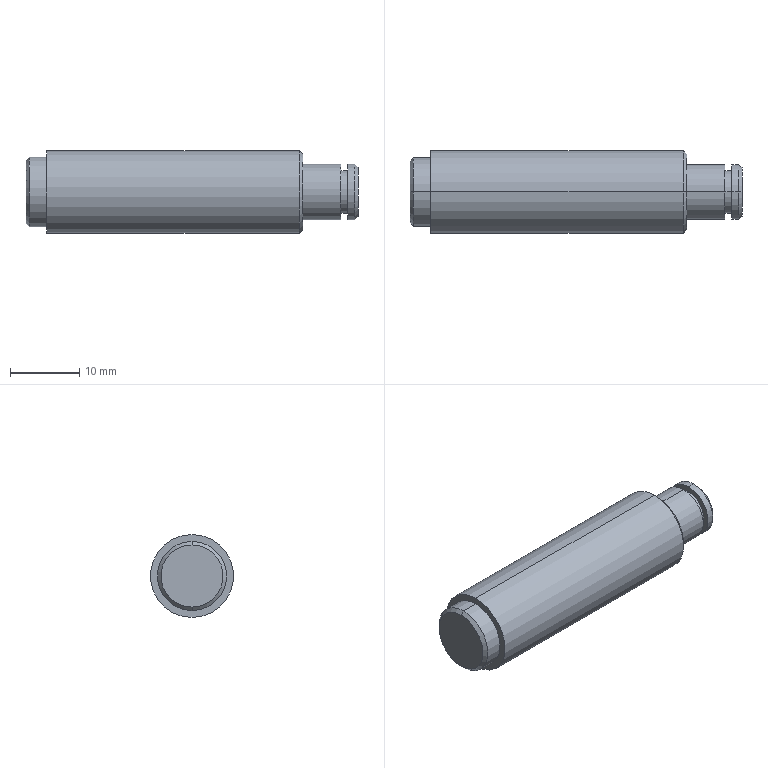Part | STEP file | 1 solid | 22 faces | box 48 x 12 x 12 mm | volume 4791 mm3 | cylinder 10 | cone 6 | plane 6 | commonest cylinder face diameters 8 x4 6.2 x2 10 x2 12 x2
STEP:
#1=CARTESIAN_POINT('',(0.,0.,0.));
#2=DIRECTION('',(0.,0.,1.));
#3=DIRECTION('',(1.,0.,0.));
#4=AXIS2_PLACEMENT_3D('',#1,#2,#3);
#5=CARTESIAN_POINT('',(3.,0.,-6.));
#6=VERTEX_POINT('',#5);
#7=CARTESIAN_POINT('',(3.,0.,6.));
#8=VERTEX_POINT('',#7);
#9=CARTESIAN_POINT('',(3.,0.,0.));
#10=DIRECTION('',(1.,0.,0.));
#11=DIRECTION('',(0.,0.,-1.));
#12=AXIS2_PLACEMENT_3D('',#9,#10,#11);
#13=CIRCLE('',#12,6.);
#14=CARTESIAN_POINT('',(21.5,0.,0.));
#15=DIRECTION('',(1.,0.,0.));
#16=DIRECTION('',(0.,0.,-1.));
#17=AXIS2_PLACEMENT_3D('',#14,#15,#16);
#18=CYLINDRICAL_SURFACE('',#17,6.);
#19=CARTESIAN_POINT('',(0.,-18.5));
#20=DIRECTION('',(1.,0.));
#21=VECTOR('',#20,1.);
#22=LINE('',#19,#21);
#23=(GEOMETRIC_REPRESENTATION_CONTEXT(2)PARAMETRIC_REPRESENTATION_CONTEXT()REPRESENTATION_CONTEXT('',''));
#24=DEFINITIONAL_REPRESENTATION('',(#22),#23);
#25=PCURVE('',#18,#24);
#26=CARTESIAN_POINT('',(3.,5.5,0.));
#27=DIRECTION('',(-1.,0.,0.));
#28=DIRECTION('',(0.,0.,1.));
#29=AXIS2_PLACEMENT_3D('',#26,#27,#28);
#30=PLANE('',#29);
#31=CARTESIAN_POINT('',(-6.,-5.5));
#32=CARTESIAN_POINT('',(-6.,4.892));
#33=CARTESIAN_POINT('',(3.,-0.3038));
#34=CARTESIAN_POINT('',(12.,-5.5));
#35=CARTESIAN_POINT('',(3.,-10.696));
#36=CARTESIAN_POINT('',(-6.,-15.892));
#37=CARTESIAN_POINT('',(-6.,-5.5));
#38=(BOUNDED_CURVE()B_SPLINE_CURVE(2,(#31,#32,#33,#34,#35,#36,#37),.UNSPECIFIED.,.T.,.F.)B_SPLINE_CURVE_WITH_KNOTS((1,2,2,2,2,1),(-2.094,0.,2.094,4.189,6.283,8.378),.UNSPECIFIED.)CURVE()GEOMETRIC_REPRESENTATION_ITEM()RATIONAL_B_SPLINE_CURVE((1.,0.5,1.,0.5,1.,0.5,1.))REPRESENTATION_ITEM(''));
#39=(GEOMETRIC_REPRESENTATION_CONTEXT(2)PARAMETRIC_REPRESENTATION_CONTEXT()REPRESENTATION_CONTEXT('',''));
#40=DEFINITIONAL_REPRESENTATION('',(#38),#39);
#41=PCURVE('',#30,#40);
#42=SURFACE_CURVE('',#13,(#25,#41),.PCURVE_S1.);
#43=EDGE_CURVE('',#6,#8,#42,.T.);
#44=ORIENTED_EDGE('',*,*,#43,.T.);
#45=CARTESIAN_POINT('',(39.5,0.,6.));
#46=VERTEX_POINT('',#45);
#47=CARTESIAN_POINT('',(21.5,0.,6.));
#48=DIRECTION('',(1.,0.,0.));
#49=VECTOR('',#48,1.);
#50=LINE('',#47,#49);
#51=CARTESIAN_POINT('',(3.142,0.));
#52=DIRECTION('',(0.,1.));
#53=VECTOR('',#52,1.);
#54=LINE('',#51,#53);
#55=(GEOMETRIC_REPRESENTATION_CONTEXT(2)PARAMETRIC_REPRESENTATION_CONTEXT()REPRESENTATION_CONTEXT('',''));
#56=DEFINITIONAL_REPRESENTATION('',(#54),#55);
#57=PCURVE('',#18,#56);
#58=CARTESIAN_POINT('',(21.5,0.,0.));
#59=DIRECTION('',(1.,0.,0.));
#60=DIRECTION('',(0.,0.,-1.));
#61=AXIS2_PLACEMENT_3D('',#58,#59,#60);
#62=CYLINDRICAL_SURFACE('',#61,6.);
#63=CARTESIAN_POINT('',(3.142,0.));
#64=DIRECTION('',(0.,1.));
#65=VECTOR('',#64,1.);
#66=LINE('',#63,#65);
#67=(GEOMETRIC_REPRESENTATION_CONTEXT(2)PARAMETRIC_REPRESENTATION_CONTEXT()REPRESENTATION_CONTEXT('',''));
#68=DEFINITIONAL_REPRESENTATION('',(#66),#67);
#69=PCURVE('',#62,#68);
#70=SURFACE_CURVE('',#50,(#57,#69),.PCURVE_S1.);
#71=EDGE_CURVE('',#8,#46,#70,.T.);
#72=ORIENTED_EDGE('',*,*,#71,.T.);
#73=CARTESIAN_POINT('',(39.5,0.,-6.));
#74=VERTEX_POINT('',#73);
#75=CARTESIAN_POINT('',(39.5,0.,0.));
#76=DIRECTION('',(-1.,0.,0.));
#77=DIRECTION('',(0.,0.,-1.));
#78=AXIS2_PLACEMENT_3D('',#75,#76,#77);
#79=CIRCLE('',#78,6.);
#80=CARTESIAN_POINT('',(6.283,18.));
#81=DIRECTION('',(-1.,0.));
#82=VECTOR('',#81,1.);
#83=LINE('',#80,#82);
#84=(GEOMETRIC_REPRESENTATION_CONTEXT(2)PARAMETRIC_REPRESENTATION_CONTEXT()REPRESENTATION_CONTEXT('',''));
#85=DEFINITIONAL_REPRESENTATION('',(#83),#84);
#86=PCURVE('',#18,#85);
#87=CARTESIAN_POINT('',(39.5,0.,0.));
#88=DIRECTION('',(-1.,0.,0.));
#89=DIRECTION('',(0.,0.,1.));
#90=AXIS2_PLACEMENT_3D('',#87,#88,#89);
#91=CONICAL_SURFACE('',#90,6.,0.7854);
#92=CARTESIAN_POINT('',(-3.142,0.));
#93=DIRECTION('',(1.,0.));
#94=VECTOR('',#93,1.);
#95=LINE('',#92,#94);
#96=(GEOMETRIC_REPRESENTATION_CONTEXT(2)PARAMETRIC_REPRESENTATION_CONTEXT()REPRESENTATION_CONTEXT('',''));
#97=DEFINITIONAL_REPRESENTATION('',(#95),#96);
#98=PCURVE('',#91,#97);
#99=SURFACE_CURVE('',#79,(#86,#98),.PCURVE_S1.);
#100=EDGE_CURVE('',#46,#74,#99,.T.);
#101=ORIENTED_EDGE('',*,*,#100,.T.);
#102=CARTESIAN_POINT('',(21.5,0.,-6.));
#103=DIRECTION('',(1.,0.,0.));
#104=VECTOR('',#103,1.);
#105=LINE('',#102,#104);
#106=CARTESIAN_POINT('',(0.,0.));
#107=DIRECTION('',(0.,1.));
#108=VECTOR('',#107,1.);
#109=LINE('',#106,#108);
#110=(GEOMETRIC_REPRESENTATION_CONTEXT(2)PARAMETRIC_REPRESENTATION_CONTEXT()REPRESENTATION_CONTEXT('',''));
#111=DEFINITIONAL_REPRESENTATION('',(#109),#110);
#112=PCURVE('',#18,#111);
#113=CARTESIAN_POINT('',(6.283,0.));
#114=DIRECTION('',(0.,1.));
#115=VECTOR('',#114,1.);
#116=LINE('',#113,#115);
#117=(GEOMETRIC_REPRESENTATION_CONTEXT(2)PARAMETRIC_REPRESENTATION_CONTEXT()REPRESENTATION_CONTEXT('',''));
#118=DEFINITIONAL_REPRESENTATION('',(#116),#117);
#119=PCURVE('',#62,#118);
#120=SURFACE_CURVE('',#105,(#112,#119),.PCURVE_S1.);
#121=EDGE_CURVE('',#6,#74,#120,.T.);
#122=ORIENTED_EDGE('',*,*,#121,.F.);
#123=EDGE_LOOP('',(#44,#72,#101,#122));
#124=FACE_BOUND('',#123,.T.);
#125=ADVANCED_FACE('',(#124),#18,.T.);
#126=CARTESIAN_POINT('',(40.,0.,5.5));
#127=VERTEX_POINT('',#126);
#128=CARTESIAN_POINT('',(40.,0.,-5.5));
#129=VERTEX_POINT('',#128);
#130=CARTESIAN_POINT('',(40.,0.,0.));
#131=DIRECTION('',(-1.,0.,0.));
#132=DIRECTION('',(0.,0.,1.));
#133=AXIS2_PLACEMENT_3D('',#130,#131,#132);
#134=CIRCLE('',#133,5.5);
#135=CARTESIAN_POINT('',(0.,-0.5));
#136=DIRECTION('',(1.,0.));
#137=VECTOR('',#136,1.);
#138=LINE('',#135,#137);
#139=(GEOMETRIC_REPRESENTATION_CONTEXT(2)PARAMETRIC_REPRESENTATION_CONTEXT()REPRESENTATION_CONTEXT('',''));
#140=DEFINITIONAL_REPRESENTATION('',(#138),#139);
#141=PCURVE('',#91,#140);
#142=CARTESIAN_POINT('',(40.,5.,0.));
#143=DIRECTION('',(1.,0.,0.));
#144=DIRECTION('',(0.,0.,-1.));
#145=AXIS2_PLACEMENT_3D('',#142,#143,#144);
#146=PLANE('',#145);
#147=CARTESIAN_POINT('',(-5.5,-5.));
#148=CARTESIAN_POINT('',(-5.5,4.526));
#149=CARTESIAN_POINT('',(2.75,-0.2369));
#150=CARTESIAN_POINT('',(11.,-5.));
#151=CARTESIAN_POINT('',(2.75,-9.763));
#152=CARTESIAN_POINT('',(-5.5,-14.526));
#153=CARTESIAN_POINT('',(-5.5,-5.));
#154=(BOUNDED_CURVE()B_SPLINE_CURVE(2,(#147,#148,#149,#150,#151,#152,#153),.UNSPECIFIED.,.T.,.F.)B_SPLINE_CURVE_WITH_KNOTS((1,2,2,2,2,1),(-2.094,0.,2.094,4.189,6.283,8.378),.UNSPECIFIED.)CURVE()GEOMETRIC_REPRESENTATION_ITEM()RATIONAL_B_SPLINE_CURVE((1.,0.5,1.,0.5,1.,0.5,1.))REPRESENTATION_ITEM(''));
#155=(GEOMETRIC_REPRESENTATION_CONTEXT(2)PARAMETRIC_REPRESENTATION_CONTEXT()REPRESENTATION_CONTEXT('',''));
#156=DEFINITIONAL_REPRESENTATION('',(#154),#155);
#157=PCURVE('',#146,#156);
#158=SURFACE_CURVE('',#134,(#141,#157),.PCURVE_S1.);
#159=EDGE_CURVE('',#127,#129,#158,.T.);
#160=ORIENTED_EDGE('',*,*,#159,.T.);
#161=CARTESIAN_POINT('',(39.5,0.,-6.));
#162=DIRECTION('',(-0.7071,0.,-0.7071));
#163=VECTOR('',#162,1.);
#164=LINE('',#161,#163);
#165=CARTESIAN_POINT('',(3.142,0.));
#166=DIRECTION('',(0.,1.));
#167=VECTOR('',#166,1.);
#168=LINE('',#165,#167);
#169=(GEOMETRIC_REPRESENTATION_CONTEXT(2)PARAMETRIC_REPRESENTATION_CONTEXT()REPRESENTATION_CONTEXT('',''));
#170=DEFINITIONAL_REPRESENTATION('',(#168),#169);
#171=PCURVE('',#91,#170);
#172=CARTESIAN_POINT('',(39.5,0.,0.));
#173=DIRECTION('',(-1.,0.,0.));
#174=DIRECTION('',(0.,0.,1.));
#175=AXIS2_PLACEMENT_3D('',#172,#173,#174);
#176=CONICAL_SURFACE('',#175,6.,0.7854);
#177=CARTESIAN_POINT('',(3.142,0.));
#178=DIRECTION('',(0.,1.));
#179=VECTOR('',#178,1.);
#180=LINE('',#177,#179);
#181=(GEOMETRIC_REPRESENTATION_CONTEXT(2)PARAMETRIC_REPRESENTATION_CONTEXT()REPRESENTATION_CONTEXT('',''));
#182=DEFINITIONAL_REPRESENTATION('',(#180),#181);
#183=PCURVE('',#176,#182);
#184=SURFACE_CURVE('',#164,(#171,#183),.PCURVE_S1.);
#185=EDGE_CURVE('',#129,#74,#184,.T.);
#186=ORIENTED_EDGE('',*,*,#185,.T.);
#187=ORIENTED_EDGE('',*,*,#100,.F.);
#188=CARTESIAN_POINT('',(39.5,0.,6.));
#189=DIRECTION('',(-0.7071,0.,0.7071));
#190=VECTOR('',#189,1.);
#191=LINE('',#188,#190);
#192=CARTESIAN_POINT('',(0.,0.));
#193=DIRECTION('',(0.,1.));
#194=VECTOR('',#193,1.);
#195=LINE('',#192,#194);
#196=(GEOMETRIC_REPRESENTATION_CONTEXT(2)PARAMETRIC_REPRESENTATION_CONTEXT()REPRESENTATION_CONTEXT('',''));
#197=DEFINITIONAL_REPRESENTATION('',(#195),#196);
#198=PCURVE('',#91,#197);
#199=CARTESIAN_POINT('',(6.283,0.));
#200=DIRECTION('',(0.,1.));
#201=VECTOR('',#200,1.);
#202=LINE('',#199,#201);
#203=(GEOMETRIC_REPRESENTATION_CONTEXT(2)PARAMETRIC_REPRESENTATION_CONTEXT()REPRESENTATION_CONTEXT('',''));
#204=DEFINITIONAL_REPRESENTATION('',(#202),#203);
#205=PCURVE('',#176,#204);
#206=SURFACE_CURVE('',#191,(#198,#205),.PCURVE_S1.);
#207=EDGE_CURVE('',#127,#46,#206,.T.);
#208=ORIENTED_EDGE('',*,*,#207,.F.);
#209=EDGE_LOOP('',(#160,#186,#187,#208));
#210=FACE_BOUND('',#209,.T.);
#211=ADVANCED_FACE('',(#210),#91,.T.);
#212=CARTESIAN_POINT('',(0.5,0.,-5.));
#213=VERTEX_POINT('',#212);
#214=CARTESIAN_POINT('',(0.5,0.,5.));
#215=VERTEX_POINT('',#214);
#216=CARTESIAN_POINT('',(0.5,0.,0.));
#217=DIRECTION('',(1.,0.,0.));
#218=DIRECTION('',(0.,0.,-1.));
#219=AXIS2_PLACEMENT_3D('',#216,#217,#218);
#220=CIRCLE('',#219,5.);
#221=CARTESIAN_POINT('',(1.5,0.,0.));
#222=DIRECTION('',(1.,0.,0.));
#223=DIRECTION('',(0.,0.,-1.));
#224=AXIS2_PLACEMENT_3D('',#221,#222,#223);
#225=CYLINDRICAL_SURFACE('',#224,5.);
#226=CARTESIAN_POINT('',(0.,-1.));
#227=DIRECTION('',(1.,0.));
#228=VECTOR('',#227,1.);
#229=LINE('',#226,#228);
#230=(GEOMETRIC_REPRESENTATION_CONTEXT(2)PARAMETRIC_REPRESENTATION_CONTEXT()REPRESENTATION_CONTEXT('',''));
#231=DEFINITIONAL_REPRESENTATION('',(#229),#230);
#232=PCURVE('',#225,#231);
#233=CARTESIAN_POINT('',(0.5,0.,0.));
#234=DIRECTION('',(1.,0.,0.));
#235=DIRECTION('',(0.,0.,-1.));
#236=AXIS2_PLACEMENT_3D('',#233,#234,#235);
#237=CONICAL_SURFACE('',#236,5.,0.7854);
#238=CARTESIAN_POINT('',(0.,0.));
#239=DIRECTION('',(1.,0.));
#240=VECTOR('',#239,1.);
#241=LINE('',#238,#240);
#242=(GEOMETRIC_REPRESENTATION_CONTEXT(2)PARAMETRIC_REPRESENTATION_CONTEXT()REPRESENTATION_CONTEXT('',''));
#243=DEFINITIONAL_REPRESENTATION('',(#241),#242);
#244=PCURVE('',#237,#243);
#245=SURFACE_CURVE('',#220,(#232,#244),.PCURVE_S1.);
#246=EDGE_CURVE('',#213,#215,#245,.T.);
#247=ORIENTED_EDGE('',*,*,#246,.T.);
#248=CARTESIAN_POINT('',(3.,0.,5.));
#249=VERTEX_POINT('',#248);
#250=CARTESIAN_POINT('',(1.5,0.,5.));
#251=DIRECTION('',(1.,0.,0.));
#252=VECTOR('',#251,1.);
#253=LINE('',#250,#252);
#254=CARTESIAN_POINT('',(3.142,0.));
#255=DIRECTION('',(0.,1.));
#256=VECTOR('',#255,1.);
#257=LINE('',#254,#256);
#258=(GEOMETRIC_REPRESENTATION_CONTEXT(2)PARAMETRIC_REPRESENTATION_CONTEXT()REPRESENTATION_CONTEXT('',''));
#259=DEFINITIONAL_REPRESENTATION('',(#257),#258);
#260=PCURVE('',#225,#259);
#261=CARTESIAN_POINT('',(1.5,0.,0.));
#262=DIRECTION('',(1.,0.,0.));
#263=DIRECTION('',(0.,0.,-1.));
#264=AXIS2_PLACEMENT_3D('',#261,#262,#263);
#265=CYLINDRICAL_SURFACE('',#264,5.);
#266=CARTESIAN_POINT('',(3.142,0.));
#267=DIRECTION('',(0.,1.));
#268=VECTOR('',#267,1.);
#269=LINE('',#266,#268);
#270=(GEOMETRIC_REPRESENTATION_CONTEXT(2)PARAMETRIC_REPRESENTATION_CONTEXT()REPRESENTATION_CONTEXT('',''));
#271=DEFINITIONAL_REPRESENTATION('',(#269),#270);
#272=PCURVE('',#265,#271);
#273=SURFACE_CURVE('',#253,(#260,#272),.PCURVE_S1.);
#274=EDGE_CURVE('',#215,#249,#273,.T.);
#275=ORIENTED_EDGE('',*,*,#274,.T.);
#276=CARTESIAN_POINT('',(3.,0.,-5.));
#277=VERTEX_POINT('',#276);
#278=CARTESIAN_POINT('',(3.,0.,0.));
#279=DIRECTION('',(1.,0.,0.));
#280=DIRECTION('',(0.,0.,-1.));
#281=AXIS2_PLACEMENT_3D('',#278,#279,#280);
#282=CIRCLE('',#281,5.);
#283=CARTESIAN_POINT('',(0.,1.5));
#284=DIRECTION('',(1.,0.));
#285=VECTOR('',#284,1.);
#286=LINE('',#283,#285);
#287=(GEOMETRIC_REPRESENTATION_CONTEXT(2)PARAMETRIC_REPRESENTATION_CONTEXT()REPRESENTATION_CONTEXT('',''));
#288=DEFINITIONAL_REPRESENTATION('',(#286),#287);
#289=PCURVE('',#225,#288);
#290=CARTESIAN_POINT('',(-5.,-5.5));
#291=CARTESIAN_POINT('',(-5.,3.16));
#292=CARTESIAN_POINT('',(2.5,-1.17));
#293=CARTESIAN_POINT('',(10.,-5.5));
#294=CARTESIAN_POINT('',(2.5,-9.83));
#295=CARTESIAN_POINT('',(-5.,-14.16));
#296=CARTESIAN_POINT('',(-5.,-5.5));
#297=(BOUNDED_CURVE()B_SPLINE_CURVE(2,(#290,#291,#292,#293,#294,#295,#296),.UNSPECIFIED.,.T.,.F.)B_SPLINE_CURVE_WITH_KNOTS((1,2,2,2,2,1),(-2.094,0.,2.094,4.189,6.283,8.378),.UNSPECIFIED.)CURVE()GEOMETRIC_REPRESENTATION_ITEM()RATIONAL_B_SPLINE_CURVE((1.,0.5,1.,0.5,1.,0.5,1.))REPRESENTATION_ITEM(''));
#298=(GEOMETRIC_REPRESENTATION_CONTEXT(2)PARAMETRIC_REPRESENTATION_CONTEXT()REPRESENTATION_CONTEXT('',''));
#299=DEFINITIONAL_REPRESENTATION('',(#297),#298);
#300=PCURVE('',#30,#299);
#301=SURFACE_CURVE('',#282,(#289,#300),.PCURVE_S1.);
#302=EDGE_CURVE('',#277,#249,#301,.T.);
#303=ORIENTED_EDGE('',*,*,#302,.F.);
#304=CARTESIAN_POINT('',(1.5,0.,-5.));
#305=DIRECTION('',(1.,0.,0.));
#306=VECTOR('',#305,1.);
#307=LINE('',#304,#306);
#308=CARTESIAN_POINT('',(0.,0.));
#309=DIRECTION('',(0.,1.));
#310=VECTOR('',#309,1.);
#311=LINE('',#308,#310);
#312=(GEOMETRIC_REPRESENTATION_CONTEXT(2)PARAMETRIC_REPRESENTATION_CONTEXT()REPRESENTATION_CONTEXT('',''));
#313=DEFINITIONAL_REPRESENTATION('',(#311),#312);
#314=PCURVE('',#225,#313);
#315=CARTESIAN_POINT('',(6.283,0.));
#316=DIRECTION('',(0.,1.));
#317=VECTOR('',#316,1.);
#318=LINE('',#315,#317);
#319=(GEOMETRIC_REPRESENTATION_CONTEXT(2)PARAMETRIC_REPRESENTATION_CONTEXT()REPRESENTATION_CONTEXT('',''));
#320=DEFINITIONAL_REPRESENTATION('',(#318),#319);
#321=PCURVE('',#265,#320);
#322=SURFACE_CURVE('',#307,(#314,#321),.PCURVE_S1.);
#323=EDGE_CURVE('',#213,#277,#322,.T.);
#324=ORIENTED_EDGE('',*,*,#323,.F.);
#325=EDGE_LOOP('',(#247,#275,#303,#324));
#326=FACE_BOUND('',#325,.T.);
#327=ADVANCED_FACE('',(#326),#225,.T.);
#328=CARTESIAN_POINT('',(40.,0.,4.));
#329=VERTEX_POINT('',#328);
#330=CARTESIAN_POINT('',(40.,0.,-4.));
#331=VERTEX_POINT('',#330);
#332=CARTESIAN_POINT('',(40.,0.,0.));
#333=DIRECTION('',(-1.,0.,0.));
#334=DIRECTION('',(0.,0.,-1.));
#335=AXIS2_PLACEMENT_3D('',#332,#333,#334);
#336=CIRCLE('',#335,4.);
#337=CARTESIAN_POINT('',(42.75,0.,0.));
#338=DIRECTION('',(1.,0.,0.));
#339=DIRECTION('',(0.,0.,-1.));
#340=AXIS2_PLACEMENT_3D('',#337,#338,#339);
#341=CYLINDRICAL_SURFACE('',#340,4.);
#342=CARTESIAN_POINT('',(6.283,-2.75));
#343=DIRECTION('',(-1.,0.));
#344=VECTOR('',#343,1.);
#345=LINE('',#342,#344);
#346=(GEOMETRIC_REPRESENTATION_CONTEXT(2)PARAMETRIC_REPRESENTATION_CONTEXT()REPRESENTATION_CONTEXT('',''));
#347=DEFINITIONAL_REPRESENTATION('',(#345),#346);
#348=PCURVE('',#341,#347);
#349=CARTESIAN_POINT('',(4.,-5.));
#350=CARTESIAN_POINT('',(4.,-11.928));
#351=CARTESIAN_POINT('',(-2.,-8.464));
#352=CARTESIAN_POINT('',(-8.,-5.));
#353=CARTESIAN_POINT('',(-2.,-1.536));
#354=CARTESIAN_POINT('',(4.,1.928));
#355=CARTESIAN_POINT('',(4.,-5.));
#356=(BOUNDED_CURVE()B_SPLINE_CURVE(2,(#349,#350,#351,#352,#353,#354,#355),.UNSPECIFIED.,.T.,.F.)B_SPLINE_CURVE_WITH_KNOTS((1,2,2,2,2,1),(-2.094,0.,2.094,4.189,6.283,8.378),.UNSPECIFIED.)CURVE()GEOMETRIC_REPRESENTATION_ITEM()RATIONAL_B_SPLINE_CURVE((1.,0.5,1.,0.5,1.,0.5,1.))REPRESENTATION_ITEM(''));
#357=(GEOMETRIC_REPRESENTATION_CONTEXT(2)PARAMETRIC_REPRESENTATION_CONTEXT()REPRESENTATION_CONTEXT('',''));
#358=DEFINITIONAL_REPRESENTATION('',(#356),#357);
#359=PCURVE('',#146,#358);
#360=SURFACE_CURVE('',#336,(#348,#359),.PCURVE_S1.);
#361=EDGE_CURVE('',#329,#331,#360,.T.);
#362=ORIENTED_EDGE('',*,*,#361,.F.);
#363=CARTESIAN_POINT('',(45.5,0.,4.));
#364=VERTEX_POINT('',#363);
#365=CARTESIAN_POINT('',(42.75,0.,4.));
#366=DIRECTION('',(1.,0.,0.));
#367=VECTOR('',#366,1.);
#368=LINE('',#365,#367);
#369=CARTESIAN_POINT('',(3.142,0.));
#370=DIRECTION('',(0.,1.));
#371=VECTOR('',#370,1.);
#372=LINE('',#369,#371);
#373=(GEOMETRIC_REPRESENTATION_CONTEXT(2)PARAMETRIC_REPRESENTATION_CONTEXT()REPRESENTATION_CONTEXT('',''));
#374=DEFINITIONAL_REPRESENTATION('',(#372),#373);
#375=PCURVE('',#341,#374);
#376=CARTESIAN_POINT('',(42.75,0.,0.));
#377=DIRECTION('',(1.,0.,0.));
#378=DIRECTION('',(0.,0.,-1.));
#379=AXIS2_PLACEMENT_3D('',#376,#377,#378);
#380=CYLINDRICAL_SURFACE('',#379,4.);
#381=CARTESIAN_POINT('',(3.142,0.));
#382=DIRECTION('',(0.,1.));
#383=VECTOR('',#382,1.);
#384=LINE('',#381,#383);
#385=(GEOMETRIC_REPRESENTATION_CONTEXT(2)PARAMETRIC_REPRESENTATION_CONTEXT()REPRESENTATION_CONTEXT('',''));
#386=DEFINITIONAL_REPRESENTATION('',(#384),#385);
#387=PCURVE('',#380,#386);
#388=SURFACE_CURVE('',#368,(#375,#387),.PCURVE_S1.);
#389=EDGE_CURVE('',#329,#364,#388,.T.);
#390=ORIENTED_EDGE('',*,*,#389,.T.);
#391=CARTESIAN_POINT('',(45.5,0.,-4.));
#392=VERTEX_POINT('',#391);
#393=CARTESIAN_POINT('',(45.5,0.,0.));
#394=DIRECTION('',(-1.,0.,0.));
#395=DIRECTION('',(0.,0.,-1.));
#396=AXIS2_PLACEMENT_3D('',#393,#394,#395);
#397=CIRCLE('',#396,4.);
#398=CARTESIAN_POINT('',(6.283,2.75));
#399=DIRECTION('',(-1.,0.));
#400=VECTOR('',#399,1.);
#401=LINE('',#398,#400);
#402=(GEOMETRIC_REPRESENTATION_CONTEXT(2)PARAMETRIC_REPRESENTATION_CONTEXT()REPRESENTATION_CONTEXT('',''));
#403=DEFINITIONAL_REPRESENTATION('',(#401),#402);
#404=PCURVE('',#341,#403);
#405=CARTESIAN_POINT('',(45.5,3.55,0.));
#406=DIRECTION('',(1.,0.,0.));
#407=DIRECTION('',(0.,0.,-1.));
#408=AXIS2_PLACEMENT_3D('',#405,#406,#407);
#409=PLANE('',#408);
#410=CARTESIAN_POINT('',(4.,-3.55));
#411=CARTESIAN_POINT('',(4.,-10.478));
#412=CARTESIAN_POINT('',(-2.,-7.014));
#413=CARTESIAN_POINT('',(-8.,-3.55));
#414=CARTESIAN_POINT('',(-2.,-0.0859));
#415=CARTESIAN_POINT('',(4.,3.378));
#416=CARTESIAN_POINT('',(4.,-3.55));
#417=(BOUNDED_CURVE()B_SPLINE_CURVE(2,(#410,#411,#412,#413,#414,#415,#416),.UNSPECIFIED.,.T.,.F.)B_SPLINE_CURVE_WITH_KNOTS((1,2,2,2,2,1),(-2.094,0.,2.094,4.189,6.283,8.378),.UNSPECIFIED.)CURVE()GEOMETRIC_REPRESENTATION_ITEM()RATIONAL_B_SPLINE_CURVE((1.,0.5,1.,0.5,1.,0.5,1.))REPRESENTATION_ITEM(''));
#418=(GEOMETRIC_REPRESENTATION_CONTEXT(2)PARAMETRIC_REPRESENTATION_CONTEXT()REPRESENTATION_CONTEXT('',''));
#419=DEFINITIONAL_REPRESENTATION('',(#417),#418);
#420=PCURVE('',#409,#419);
#421=SURFACE_CURVE('',#397,(#404,#420),.PCURVE_S1.);
#422=EDGE_CURVE('',#364,#392,#421,.T.);
#423=ORIENTED_EDGE('',*,*,#422,.T.);
#424=CARTESIAN_POINT('',(42.75,0.,-4.));
#425=DIRECTION('',(1.,0.,0.));
#426=VECTOR('',#425,1.);
#427=LINE('',#424,#426);
#428=CARTESIAN_POINT('',(0.,0.));
#429=DIRECTION('',(0.,1.));
#430=VECTOR('',#429,1.);
#431=LINE('',#428,#430);
#432=(GEOMETRIC_REPRESENTATION_CONTEXT(2)PARAMETRIC_REPRESENTATION_CONTEXT()REPRESENTATION_CONTEXT('',''));
#433=DEFINITIONAL_REPRESENTATION('',(#431),#432);
#434=PCURVE('',#341,#433);
#435=CARTESIAN_POINT('',(6.283,0.));
#436=DIRECTION('',(0.,1.));
#437=VECTOR('',#436,1.);
#438=LINE('',#435,#437);
#439=(GEOMETRIC_REPRESENTATION_CONTEXT(2)PARAMETRIC_REPRESENTATION_CONTEXT()REPRESENTATION_CONTEXT('',''));
#440=DEFINITIONAL_REPRESENTATION('',(#438),#439);
#441=PCURVE('',#380,#440);
#442=SURFACE_CURVE('',#427,(#434,#441),.PCURVE_S1.);
#443=EDGE_CURVE('',#331,#392,#442,.T.);
#444=ORIENTED_EDGE('',*,*,#443,.F.);
#445=EDGE_LOOP('',(#362,#390,#423,#444));
#446=FACE_BOUND('',#445,.T.);
#447=ADVANCED_FACE('',(#446),#341,.T.);
#448=CARTESIAN_POINT('',(0.,0.,-4.5));
#449=VERTEX_POINT('',#448);
#450=CARTESIAN_POINT('',(0.,0.,4.5));
#451=VERTEX_POINT('',#450);
#452=CARTESIAN_POINT('',(0.,0.,0.));
#453=DIRECTION('',(1.,0.,0.));
#454=DIRECTION('',(0.,0.,-1.));
#455=AXIS2_PLACEMENT_3D('',#452,#453,#454);
#456=CIRCLE('',#455,4.5);
#457=CARTESIAN_POINT('',(0.,-0.5));
#458=DIRECTION('',(1.,0.));
#459=VECTOR('',#458,1.);
#460=LINE('',#457,#459);
#461=(GEOMETRIC_REPRESENTATION_CONTEXT(2)PARAMETRIC_REPRESENTATION_CONTEXT()REPRESENTATION_CONTEXT('',''));
#462=DEFINITIONAL_REPRESENTATION('',(#460),#461);
#463=PCURVE('',#237,#462);
#464=CARTESIAN_POINT('',(0.,2.5,0.));
#465=DIRECTION('',(-1.,0.,0.));
#466=DIRECTION('',(0.,0.,1.));
#467=AXIS2_PLACEMENT_3D('',#464,#465,#466);
#468=PLANE('',#467);
#469=CARTESIAN_POINT('',(-4.5,-2.5));
#470=CARTESIAN_POINT('',(-4.5,5.294));
#471=CARTESIAN_POINT('',(2.25,1.397));
#472=CARTESIAN_POINT('',(9.,-2.5));
#473=CARTESIAN_POINT('',(2.25,-6.397));
#474=CARTESIAN_POINT('',(-4.5,-10.294));
#475=CARTESIAN_POINT('',(-4.5,-2.5));
#476=(BOUNDED_CURVE()B_SPLINE_CURVE(2,(#469,#470,#471,#472,#473,#474,#475),.UNSPECIFIED.,.T.,.F.)B_SPLINE_CURVE_WITH_KNOTS((1,2,2,2,2,1),(-2.094,0.,2.094,4.189,6.283,8.378),.UNSPECIFIED.)CURVE()GEOMETRIC_REPRESENTATION_ITEM()RATIONAL_B_SPLINE_CURVE((1.,0.5,1.,0.5,1.,0.5,1.))REPRESENTATION_ITEM(''));
#477=(GEOMETRIC_REPRESENTATION_CONTEXT(2)PARAMETRIC_REPRESENTATION_CONTEXT()REPRESENTATION_CONTEXT('',''));
#478=DEFINITIONAL_REPRESENTATION('',(#476),#477);
#479=PCURVE('',#468,#478);
#480=SURFACE_CURVE('',#456,(#463,#479),.PCURVE_S1.);
#481=EDGE_CURVE('',#449,#451,#480,.T.);
#482=ORIENTED_EDGE('',*,*,#481,.T.);
#483=CARTESIAN_POINT('',(0.5,0.,5.));
#484=DIRECTION('',(0.7071,0.,0.7071));
#485=VECTOR('',#484,1.);
#486=LINE('',#483,#485);
#487=CARTESIAN_POINT('',(3.142,0.));
#488=DIRECTION('',(0.,1.));
#489=VECTOR('',#488,1.);
#490=LINE('',#487,#489);
#491=(GEOMETRIC_REPRESENTATION_CONTEXT(2)PARAMETRIC_REPRESENTATION_CONTEXT()REPRESENTATION_CONTEXT('',''));
#492=DEFINITIONAL_REPRESENTATION('',(#490),#491);
#493=PCURVE('',#237,#492);
#494=CARTESIAN_POINT('',(0.5,0.,0.));
#495=DIRECTION('',(1.,0.,0.));
#496=DIRECTION('',(0.,0.,-1.));
#497=AXIS2_PLACEMENT_3D('',#494,#495,#496);
#498=CONICAL_SURFACE('',#497,5.,0.7854);
#499=CARTESIAN_POINT('',(3.142,0.));
#500=DIRECTION('',(0.,1.));
#501=VECTOR('',#500,1.);
#502=LINE('',#499,#501);
#503=(GEOMETRIC_REPRESENTATION_CONTEXT(2)PARAMETRIC_REPRESENTATION_CONTEXT()REPRESENTATION_CONTEXT('',''));
#504=DEFINITIONAL_REPRESENTATION('',(#502),#503);
#505=PCURVE('',#498,#504);
#506=SURFACE_CURVE('',#486,(#493,#505),.PCURVE_S1.);
#507=EDGE_CURVE('',#451,#215,#506,.T.);
#508=ORIENTED_EDGE('',*,*,#507,.T.);
#509=ORIENTED_EDGE('',*,*,#246,.F.);
#510=CARTESIAN_POINT('',(0.5,0.,-5.));
#511=DIRECTION('',(0.7071,0.,-0.7071));
#512=VECTOR('',#511,1.);
#513=LINE('',#510,#512);
#514=CARTESIAN_POINT('',(0.,0.));
#515=DIRECTION('',(0.,1.));
#516=VECTOR('',#515,1.);
#517=LINE('',#514,#516);
#518=(GEOMETRIC_REPRESENTATION_CONTEXT(2)PARAMETRIC_REPRESENTATION_CONTEXT()REPRESENTATION_CONTEXT('',''));
#519=DEFINITIONAL_REPRESENTATION('',(#517),#518);
#520=PCURVE('',#237,#519);
#521=CARTESIAN_POINT('',(6.283,0.));
#522=DIRECTION('',(0.,1.));
#523=VECTOR('',#522,1.);
#524=LINE('',#521,#523);
#525=(GEOMETRIC_REPRESENTATION_CONTEXT(2)PARAMETRIC_REPRESENTATION_CONTEXT()REPRESENTATION_CONTEXT('',''));
#526=DEFINITIONAL_REPRESENTATION('',(#524),#525);
#527=PCURVE('',#498,#526);
#528=SURFACE_CURVE('',#513,(#520,#527),.PCURVE_S1.);
#529=EDGE_CURVE('',#449,#213,#528,.T.);
#530=ORIENTED_EDGE('',*,*,#529,.F.);
#531=EDGE_LOOP('',(#482,#508,#509,#530));
#532=FACE_BOUND('',#531,.T.);
#533=ADVANCED_FACE('',(#532),#237,.T.);
#534=CARTESIAN_POINT('',(45.5,0.,3.1));
#535=VERTEX_POINT('',#534);
#536=CARTESIAN_POINT('',(45.5,0.,-3.1));
#537=VERTEX_POINT('',#536);
#538=CARTESIAN_POINT('',(45.5,0.,0.));
#539=DIRECTION('',(-1.,0.,0.));
#540=DIRECTION('',(0.,0.,-1.));
#541=AXIS2_PLACEMENT_3D('',#538,#539,#540);
#542=CIRCLE('',#541,3.1);
#543=CARTESIAN_POINT('',(46.,0.,0.));
#544=DIRECTION('',(1.,0.,0.));
#545=DIRECTION('',(0.,0.,-1.));
#546=AXIS2_PLACEMENT_3D('',#543,#544,#545);
#547=CYLINDRICAL_SURFACE('',#546,3.1);
#548=CARTESIAN_POINT('',(6.283,-0.5));
#549=DIRECTION('',(-1.,0.));
#550=VECTOR('',#549,1.);
#551=LINE('',#548,#550);
#552=(GEOMETRIC_REPRESENTATION_CONTEXT(2)PARAMETRIC_REPRESENTATION_CONTEXT()REPRESENTATION_CONTEXT('',''));
#553=DEFINITIONAL_REPRESENTATION('',(#551),#552);
#554=PCURVE('',#547,#553);
#555=CARTESIAN_POINT('',(3.1,-3.55));
#556=CARTESIAN_POINT('',(3.1,-8.919));
#557=CARTESIAN_POINT('',(-1.55,-6.235));
#558=CARTESIAN_POINT('',(-6.2,-3.55));
#559=CARTESIAN_POINT('',(-1.55,-0.8653));
#560=CARTESIAN_POINT('',(3.1,1.819));
#561=CARTESIAN_POINT('',(3.1,-3.55));
#562=(BOUNDED_CURVE()B_SPLINE_CURVE(2,(#555,#556,#557,#558,#559,#560,#561),.UNSPECIFIED.,.T.,.F.)B_SPLINE_CURVE_WITH_KNOTS((1,2,2,2,2,1),(-2.094,0.,2.094,4.189,6.283,8.378),.UNSPECIFIED.)CURVE()GEOMETRIC_REPRESENTATION_ITEM()RATIONAL_B_SPLINE_CURVE((1.,0.5,1.,0.5,1.,0.5,1.))REPRESENTATION_ITEM(''));
#563=(GEOMETRIC_REPRESENTATION_CONTEXT(2)PARAMETRIC_REPRESENTATION_CONTEXT()REPRESENTATION_CONTEXT('',''));
#564=DEFINITIONAL_REPRESENTATION('',(#562),#563);
#565=PCURVE('',#409,#564);
#566=SURFACE_CURVE('',#542,(#554,#565),.PCURVE_S1.);
#567=EDGE_CURVE('',#535,#537,#566,.T.);
#568=ORIENTED_EDGE('',*,*,#567,.F.);
#569=CARTESIAN_POINT('',(46.5,0.,3.1));
#570=VERTEX_POINT('',#569);
#571=CARTESIAN_POINT('',(46.,0.,3.1));
#572=DIRECTION('',(1.,0.,0.));
#573=VECTOR('',#572,1.);
#574=LINE('',#571,#573);
#575=CARTESIAN_POINT('',(3.142,0.));
#576=DIRECTION('',(0.,1.));
#577=VECTOR('',#576,1.);
#578=LINE('',#575,#577);
#579=(GEOMETRIC_REPRESENTATION_CONTEXT(2)PARAMETRIC_REPRESENTATION_CONTEXT()REPRESENTATION_CONTEXT('',''));
#580=DEFINITIONAL_REPRESENTATION('',(#578),#579);
#581=PCURVE('',#547,#580);
#582=CARTESIAN_POINT('',(46.,0.,0.));
#583=DIRECTION('',(1.,0.,0.));
#584=DIRECTION('',(0.,0.,-1.));
#585=AXIS2_PLACEMENT_3D('',#582,#583,#584);
#586=CYLINDRICAL_SURFACE('',#585,3.1);
#587=CARTESIAN_POINT('',(3.142,0.));
#588=DIRECTION('',(0.,1.));
#589=VECTOR('',#588,1.);
#590=LINE('',#587,#589);
#591=(GEOMETRIC_REPRESENTATION_CONTEXT(2)PARAMETRIC_REPRESENTATION_CONTEXT()REPRESENTATION_CONTEXT('',''));
#592=DEFINITIONAL_REPRESENTATION('',(#590),#591);
#593=PCURVE('',#586,#592);
#594=SURFACE_CURVE('',#574,(#581,#593),.PCURVE_S1.);
#595=EDGE_CURVE('',#535,#570,#594,.T.);
#596=ORIENTED_EDGE('',*,*,#595,.T.);
#597=CARTESIAN_POINT('',(46.5,0.,-3.1));
#598=VERTEX_POINT('',#597);
#599=CARTESIAN_POINT('',(46.5,0.,0.));
#600=DIRECTION('',(-1.,0.,0.));
#601=DIRECTION('',(0.,0.,-1.));
#602=AXIS2_PLACEMENT_3D('',#599,#600,#601);
#603=CIRCLE('',#602,3.1);
#604=CARTESIAN_POINT('',(6.283,0.5));
#605=DIRECTION('',(-1.,0.));
#606=VECTOR('',#605,1.);
#607=LINE('',#604,#606);
#608=(GEOMETRIC_REPRESENTATION_CONTEXT(2)PARAMETRIC_REPRESENTATION_CONTEXT()REPRESENTATION_CONTEXT('',''));
#609=DEFINITIONAL_REPRESENTATION('',(#607),#608);
#610=PCURVE('',#547,#609);
#611=CARTESIAN_POINT('',(46.5,3.55,0.));
#612=DIRECTION('',(-1.,0.,0.));
#613=DIRECTION('',(0.,0.,1.));
#614=AXIS2_PLACEMENT_3D('',#611,#612,#613);
#615=PLANE('',#614);
#616=CARTESIAN_POINT('',(0.,-3.55));
#617=DIRECTION('',(-1.,0.));
#618=AXIS2_PLACEMENT_2D('',#616,#617);
#619=CIRCLE('',#618,3.1);
#620=(GEOMETRIC_REPRESENTATION_CONTEXT(2)PARAMETRIC_REPRESENTATION_CONTEXT()REPRESENTATION_CONTEXT('',''));
#621=DEFINITIONAL_REPRESENTATION('',(#619),#620);
#622=PCURVE('',#615,#621);
#623=SURFACE_CURVE('',#603,(#610,#622),.PCURVE_S1.);
#624=EDGE_CURVE('',#570,#598,#623,.T.);
#625=ORIENTED_EDGE('',*,*,#624,.T.);
#626=CARTESIAN_POINT('',(46.,0.,-3.1));
#627=DIRECTION('',(1.,0.,0.));
#628=VECTOR('',#627,1.);
#629=LINE('',#626,#628);
#630=CARTESIAN_POINT('',(0.,0.));
#631=DIRECTION('',(0.,1.));
#632=VECTOR('',#631,1.);
#633=LINE('',#630,#632);
#634=(GEOMETRIC_REPRESENTATION_CONTEXT(2)PARAMETRIC_REPRESENTATION_CONTEXT()REPRESENTATION_CONTEXT('',''));
#635=DEFINITIONAL_REPRESENTATION('',(#633),#634);
#636=PCURVE('',#547,#635);
#637=CARTESIAN_POINT('',(6.283,0.));
#638=DIRECTION('',(0.,1.));
#639=VECTOR('',#638,1.);
#640=LINE('',#637,#639);
#641=(GEOMETRIC_REPRESENTATION_CONTEXT(2)PARAMETRIC_REPRESENTATION_CONTEXT()REPRESENTATION_CONTEXT('',''));
#642=DEFINITIONAL_REPRESENTATION('',(#640),#641);
#643=PCURVE('',#586,#642);
#644=SURFACE_CURVE('',#629,(#636,#643),.PCURVE_S1.);
#645=EDGE_CURVE('',#537,#598,#644,.T.);
#646=ORIENTED_EDGE('',*,*,#645,.F.);
#647=EDGE_LOOP('',(#568,#596,#625,#646));
#648=FACE_BOUND('',#647,.T.);
#649=ADVANCED_FACE('',(#648),#547,.T.);
#650=CARTESIAN_POINT('',(46.5,0.,4.));
#651=VERTEX_POINT('',#650);
#652=CARTESIAN_POINT('',(46.5,0.,-4.));
#653=VERTEX_POINT('',#652);
#654=CARTESIAN_POINT('',(46.5,0.,0.));
#655=DIRECTION('',(-1.,0.,0.));
#656=DIRECTION('',(0.,0.,-1.));
#657=AXIS2_PLACEMENT_3D('',#654,#655,#656);
#658=CIRCLE('',#657,4.);
#659=CARTESIAN_POINT('',(47.25,0.,0.));
#660=DIRECTION('',(1.,0.,0.));
#661=DIRECTION('',(0.,0.,-1.));
#662=AXIS2_PLACEMENT_3D('',#659,#660,#661);
#663=CYLINDRICAL_SURFACE('',#662,4.);
#664=CARTESIAN_POINT('',(6.283,-0.75));
#665=DIRECTION('',(-1.,0.));
#666=VECTOR('',#665,1.);
#667=LINE('',#664,#666);
#668=(GEOMETRIC_REPRESENTATION_CONTEXT(2)PARAMETRIC_REPRESENTATION_CONTEXT()REPRESENTATION_CONTEXT('',''));
#669=DEFINITIONAL_REPRESENTATION('',(#667),#668);
#670=PCURVE('',#663,#669);
#671=CARTESIAN_POINT('',(0.,-3.55));
#672=DIRECTION('',(-1.,0.));
#673=AXIS2_PLACEMENT_2D('',#671,#672);
#674=CIRCLE('',#673,4.);
#675=(GEOMETRIC_REPRESENTATION_CONTEXT(2)PARAMETRIC_REPRESENTATION_CONTEXT()REPRESENTATION_CONTEXT('',''));
#676=DEFINITIONAL_REPRESENTATION('',(#674),#675);
#677=PCURVE('',#615,#676);
#678=SURFACE_CURVE('',#658,(#670,#677),.PCURVE_S1.);
#679=EDGE_CURVE('',#651,#653,#678,.T.);
#680=ORIENTED_EDGE('',*,*,#679,.F.);
#681=CARTESIAN_POINT('',(47.5,0.,4.));
#682=VERTEX_POINT('',#681);
#683=CARTESIAN_POINT('',(47.25,0.,4.));
#684=DIRECTION('',(1.,0.,0.));
#685=VECTOR('',#684,1.);
#686=LINE('',#683,#685);
#687=CARTESIAN_POINT('',(3.142,0.));
#688=DIRECTION('',(0.,1.));
#689=VECTOR('',#688,1.);
#690=LINE('',#687,#689);
#691=(GEOMETRIC_REPRESENTATION_CONTEXT(2)PARAMETRIC_REPRESENTATION_CONTEXT()REPRESENTATION_CONTEXT('',''));
#692=DEFINITIONAL_REPRESENTATION('',(#690),#691);
#693=PCURVE('',#663,#692);
#694=CARTESIAN_POINT('',(47.25,0.,0.));
#695=DIRECTION('',(1.,0.,0.));
#696=DIRECTION('',(0.,0.,-1.));
#697=AXIS2_PLACEMENT_3D('',#694,#695,#696);
#698=CYLINDRICAL_SURFACE('',#697,4.);
#699=CARTESIAN_POINT('',(3.142,0.));
#700=DIRECTION('',(0.,1.));
#701=VECTOR('',#700,1.);
#702=LINE('',#699,#701);
#703=(GEOMETRIC_REPRESENTATION_CONTEXT(2)PARAMETRIC_REPRESENTATION_CONTEXT()REPRESENTATION_CONTEXT('',''));
#704=DEFINITIONAL_REPRESENTATION('',(#702),#703);
#705=PCURVE('',#698,#704);
#706=SURFACE_CURVE('',#686,(#693,#705),.PCURVE_S1.);
#707=EDGE_CURVE('',#651,#682,#706,.T.);
#708=ORIENTED_EDGE('',*,*,#707,.T.);
#709=CARTESIAN_POINT('',(47.5,0.,-4.));
#710=VERTEX_POINT('',#709);
#711=CARTESIAN_POINT('',(47.5,0.,0.));
#712=DIRECTION('',(-1.,0.,0.));
#713=DIRECTION('',(0.,0.,-1.));
#714=AXIS2_PLACEMENT_3D('',#711,#712,#713);
#715=CIRCLE('',#714,4.);
#716=CARTESIAN_POINT('',(6.283,0.25));
#717=DIRECTION('',(-1.,0.));
#718=VECTOR('',#717,1.);
#719=LINE('',#716,#718);
#720=(GEOMETRIC_REPRESENTATION_CONTEXT(2)PARAMETRIC_REPRESENTATION_CONTEXT()REPRESENTATION_CONTEXT('',''));
#721=DEFINITIONAL_REPRESENTATION('',(#719),#720);
#722=PCURVE('',#663,#721);
#723=CARTESIAN_POINT('',(47.5,0.,0.));
#724=DIRECTION('',(-1.,0.,0.));
#725=DIRECTION('',(0.,0.,1.));
#726=AXIS2_PLACEMENT_3D('',#723,#724,#725);
#727=CONICAL_SURFACE('',#726,4.,0.7854);
#728=CARTESIAN_POINT('',(-3.142,0.));
#729=DIRECTION('',(1.,0.));
#730=VECTOR('',#729,1.);
#731=LINE('',#728,#730);
#732=(GEOMETRIC_REPRESENTATION_CONTEXT(2)PARAMETRIC_REPRESENTATION_CONTEXT()REPRESENTATION_CONTEXT('',''));
#733=DEFINITIONAL_REPRESENTATION('',(#731),#732);
#734=PCURVE('',#727,#733);
#735=SURFACE_CURVE('',#715,(#722,#734),.PCURVE_S1.);
#736=EDGE_CURVE('',#682,#710,#735,.T.);
#737=ORIENTED_EDGE('',*,*,#736,.T.);
#738=CARTESIAN_POINT('',(47.25,0.,-4.));
#739=DIRECTION('',(1.,0.,0.));
#740=VECTOR('',#739,1.);
#741=LINE('',#738,#740);
#742=CARTESIAN_POINT('',(0.,0.));
#743=DIRECTION('',(0.,1.));
#744=VECTOR('',#743,1.);
#745=LINE('',#742,#744);
#746=(GEOMETRIC_REPRESENTATION_CONTEXT(2)PARAMETRIC_REPRESENTATION_CONTEXT()REPRESENTATION_CONTEXT('',''));
#747=DEFINITIONAL_REPRESENTATION('',(#745),#746);
#748=PCURVE('',#663,#747);
#749=CARTESIAN_POINT('',(6.283,0.));
#750=DIRECTION('',(0.,1.));
#751=VECTOR('',#750,1.);
#752=LINE('',#749,#751);
#753=(GEOMETRIC_REPRESENTATION_CONTEXT(2)PARAMETRIC_REPRESENTATION_CONTEXT()REPRESENTATION_CONTEXT('',''));
#754=DEFINITIONAL_REPRESENTATION('',(#752),#753);
#755=PCURVE('',#698,#754);
#756=SURFACE_CURVE('',#741,(#748,#755),.PCURVE_S1.);
#757=EDGE_CURVE('',#653,#710,#756,.T.);
#758=ORIENTED_EDGE('',*,*,#757,.F.);
#759=EDGE_LOOP('',(#680,#708,#737,#758));
#760=FACE_BOUND('',#759,.T.);
#761=ADVANCED_FACE('',(#760),#663,.T.);
#762=CARTESIAN_POINT('',(48.,0.,3.5));
#763=VERTEX_POINT('',#762);
#764=CARTESIAN_POINT('',(48.,0.,-3.5));
#765=VERTEX_POINT('',#764);
#766=CARTESIAN_POINT('',(48.,0.,0.));
#767=DIRECTION('',(-1.,0.,0.));
#768=DIRECTION('',(0.,0.,1.));
#769=AXIS2_PLACEMENT_3D('',#766,#767,#768);
#770=CIRCLE('',#769,3.5);
#771=CARTESIAN_POINT('',(0.,-0.5));
#772=DIRECTION('',(1.,0.));
#773=VECTOR('',#772,1.);
#774=LINE('',#771,#773);
#775=(GEOMETRIC_REPRESENTATION_CONTEXT(2)PARAMETRIC_REPRESENTATION_CONTEXT()REPRESENTATION_CONTEXT('',''));
#776=DEFINITIONAL_REPRESENTATION('',(#774),#775);
#777=PCURVE('',#727,#776);
#778=CARTESIAN_POINT('',(48.,2.,0.));
#779=DIRECTION('',(1.,0.,0.));
#780=DIRECTION('',(0.,0.,-1.));
#781=AXIS2_PLACEMENT_3D('',#778,#779,#780);
#782=PLANE('',#781);
#783=CARTESIAN_POINT('',(-3.5,-2.));
#784=CARTESIAN_POINT('',(-3.5,4.062));
#785=CARTESIAN_POINT('',(1.75,1.031));
#786=CARTESIAN_POINT('',(7.,-2.));
#787=CARTESIAN_POINT('',(1.75,-5.031));
#788=CARTESIAN_POINT('',(-3.5,-8.062));
#789=CARTESIAN_POINT('',(-3.5,-2.));
#790=(BOUNDED_CURVE()B_SPLINE_CURVE(2,(#783,#784,#785,#786,#787,#788,#789),.UNSPECIFIED.,.T.,.F.)B_SPLINE_CURVE_WITH_KNOTS((1,2,2,2,2,1),(-2.094,0.,2.094,4.189,6.283,8.378),.UNSPECIFIED.)CURVE()GEOMETRIC_REPRESENTATION_ITEM()RATIONAL_B_SPLINE_CURVE((1.,0.5,1.,0.5,1.,0.5,1.))REPRESENTATION_ITEM(''));
#791=(GEOMETRIC_REPRESENTATION_CONTEXT(2)PARAMETRIC_REPRESENTATION_CONTEXT()REPRESENTATION_CONTEXT('',''));
#792=DEFINITIONAL_REPRESENTATION('',(#790),#791);
#793=PCURVE('',#782,#792);
#794=SURFACE_CURVE('',#770,(#777,#793),.PCURVE_S1.);
#795=EDGE_CURVE('',#763,#765,#794,.T.);
#796=ORIENTED_EDGE('',*,*,#795,.T.);
#797=CARTESIAN_POINT('',(47.5,0.,-4.));
#798=DIRECTION('',(-0.7071,0.,-0.7071));
#799=VECTOR('',#798,1.);
#800=LINE('',#797,#799);
#801=CARTESIAN_POINT('',(3.142,0.));
#802=DIRECTION('',(0.,1.));
#803=VECTOR('',#802,1.);
#804=LINE('',#801,#803);
#805=(GEOMETRIC_REPRESENTATION_CONTEXT(2)PARAMETRIC_REPRESENTATION_CONTEXT()REPRESENTATION_CONTEXT('',''));
#806=DEFINITIONAL_REPRESENTATION('',(#804),#805);
#807=PCURVE('',#727,#806);
#808=CARTESIAN_POINT('',(47.5,0.,0.));
#809=DIRECTION('',(-1.,0.,0.));
#810=DIRECTION('',(0.,0.,1.));
#811=AXIS2_PLACEMENT_3D('',#808,#809,#810);
#812=CONICAL_SURFACE('',#811,4.,0.7854);
#813=CARTESIAN_POINT('',(3.142,0.));
#814=DIRECTION('',(0.,1.));
#815=VECTOR('',#814,1.);
#816=LINE('',#813,#815);
#817=(GEOMETRIC_REPRESENTATION_CONTEXT(2)PARAMETRIC_REPRESENTATION_CONTEXT()REPRESENTATION_CONTEXT('',''));
#818=DEFINITIONAL_REPRESENTATION('',(#816),#817);
#819=PCURVE('',#812,#818);
#820=SURFACE_CURVE('',#800,(#807,#819),.PCURVE_S1.);
#821=EDGE_CURVE('',#765,#710,#820,.T.);
#822=ORIENTED_EDGE('',*,*,#821,.T.);
#823=ORIENTED_EDGE('',*,*,#736,.F.);
#824=CARTESIAN_POINT('',(47.5,0.,4.));
#825=DIRECTION('',(-0.7071,0.,0.7071));
#826=VECTOR('',#825,1.);
#827=LINE('',#824,#826);
#828=CARTESIAN_POINT('',(0.,0.));
#829=DIRECTION('',(0.,1.));
#830=VECTOR('',#829,1.);
#831=LINE('',#828,#830);
#832=(GEOMETRIC_REPRESENTATION_CONTEXT(2)PARAMETRIC_REPRESENTATION_CONTEXT()REPRESENTATION_CONTEXT('',''));
#833=DEFINITIONAL_REPRESENTATION('',(#831),#832);
#834=PCURVE('',#727,#833);
#835=CARTESIAN_POINT('',(6.283,0.));
#836=DIRECTION('',(0.,1.));
#837=VECTOR('',#836,1.);
#838=LINE('',#835,#837);
#839=(GEOMETRIC_REPRESENTATION_CONTEXT(2)PARAMETRIC_REPRESENTATION_CONTEXT()REPRESENTATION_CONTEXT('',''));
#840=DEFINITIONAL_REPRESENTATION('',(#838),#839);
#841=PCURVE('',#812,#840);
#842=SURFACE_CURVE('',#827,(#834,#841),.PCURVE_S1.);
#843=EDGE_CURVE('',#763,#682,#842,.T.);
#844=ORIENTED_EDGE('',*,*,#843,.F.);
#845=EDGE_LOOP('',(#796,#822,#823,#844));
#846=FACE_BOUND('',#845,.T.);
#847=ADVANCED_FACE('',(#846),#727,.T.);
#848=ORIENTED_EDGE('',*,*,#71,.F.);
#849=CARTESIAN_POINT('',(3.,0.,0.));
#850=DIRECTION('',(1.,0.,0.));
#851=DIRECTION('',(0.,0.,-1.));
#852=AXIS2_PLACEMENT_3D('',#849,#850,#851);
#853=CIRCLE('',#852,6.);
#854=CARTESIAN_POINT('',(0.,-18.5));
#855=DIRECTION('',(1.,0.));
#856=VECTOR('',#855,1.);
#857=LINE('',#854,#856);
#858=(GEOMETRIC_REPRESENTATION_CONTEXT(2)PARAMETRIC_REPRESENTATION_CONTEXT()REPRESENTATION_CONTEXT('',''));
#859=DEFINITIONAL_REPRESENTATION('',(#857),#858);
#860=PCURVE('',#62,#859);
#861=CARTESIAN_POINT('',(-6.,-5.5));
#862=CARTESIAN_POINT('',(-6.,4.892));
#863=CARTESIAN_POINT('',(3.,-0.3038));
#864=CARTESIAN_POINT('',(12.,-5.5));
#865=CARTESIAN_POINT('',(3.,-10.696));
#866=CARTESIAN_POINT('',(-6.,-15.892));
#867=CARTESIAN_POINT('',(-6.,-5.5));
#868=(BOUNDED_CURVE()B_SPLINE_CURVE(2,(#861,#862,#863,#864,#865,#866,#867),.UNSPECIFIED.,.T.,.F.)B_SPLINE_CURVE_WITH_KNOTS((1,2,2,2,2,1),(-2.094,0.,2.094,4.189,6.283,8.378),.UNSPECIFIED.)CURVE()GEOMETRIC_REPRESENTATION_ITEM()RATIONAL_B_SPLINE_CURVE((1.,0.5,1.,0.5,1.,0.5,1.))REPRESENTATION_ITEM(''));
#869=(GEOMETRIC_REPRESENTATION_CONTEXT(2)PARAMETRIC_REPRESENTATION_CONTEXT()REPRESENTATION_CONTEXT('',''));
#870=DEFINITIONAL_REPRESENTATION('',(#868),#869);
#871=PCURVE('',#30,#870);
#872=SURFACE_CURVE('',#853,(#860,#871),.PCURVE_S1.);
#873=EDGE_CURVE('',#8,#6,#872,.T.);
#874=ORIENTED_EDGE('',*,*,#873,.T.);
#875=ORIENTED_EDGE('',*,*,#121,.T.);
#876=CARTESIAN_POINT('',(39.5,0.,0.));
#877=DIRECTION('',(-1.,0.,0.));
#878=DIRECTION('',(0.,0.,-1.));
#879=AXIS2_PLACEMENT_3D('',#876,#877,#878);
#880=CIRCLE('',#879,6.);
#881=CARTESIAN_POINT('',(6.283,18.));
#882=DIRECTION('',(-1.,0.));
#883=VECTOR('',#882,1.);
#884=LINE('',#881,#883);
#885=(GEOMETRIC_REPRESENTATION_CONTEXT(2)PARAMETRIC_REPRESENTATION_CONTEXT()REPRESENTATION_CONTEXT('',''));
#886=DEFINITIONAL_REPRESENTATION('',(#884),#885);
#887=PCURVE('',#62,#886);
#888=CARTESIAN_POINT('',(3.142,0.));
#889=DIRECTION('',(1.,0.));
#890=VECTOR('',#889,1.);
#891=LINE('',#888,#890);
#892=(GEOMETRIC_REPRESENTATION_CONTEXT(2)PARAMETRIC_REPRESENTATION_CONTEXT()REPRESENTATION_CONTEXT('',''));
#893=DEFINITIONAL_REPRESENTATION('',(#891),#892);
#894=PCURVE('',#176,#893);
#895=SURFACE_CURVE('',#880,(#887,#894),.PCURVE_S1.);
#896=EDGE_CURVE('',#74,#46,#895,.T.);
#897=ORIENTED_EDGE('',*,*,#896,.T.);
#898=EDGE_LOOP('',(#848,#874,#875,#897));
#899=FACE_BOUND('',#898,.T.);
#900=ADVANCED_FACE('',(#899),#62,.T.);
#901=ORIENTED_EDGE('',*,*,#185,.F.);
#902=CARTESIAN_POINT('',(40.,0.,0.));
#903=DIRECTION('',(-1.,0.,0.));
#904=DIRECTION('',(0.,0.,1.));
#905=AXIS2_PLACEMENT_3D('',#902,#903,#904);
#906=CIRCLE('',#905,5.5);
#907=CARTESIAN_POINT('',(0.,-0.5));
#908=DIRECTION('',(1.,0.));
#909=VECTOR('',#908,1.);
#910=LINE('',#907,#909);
#911=(GEOMETRIC_REPRESENTATION_CONTEXT(2)PARAMETRIC_REPRESENTATION_CONTEXT()REPRESENTATION_CONTEXT('',''));
#912=DEFINITIONAL_REPRESENTATION('',(#910),#911);
#913=PCURVE('',#176,#912);
#914=CARTESIAN_POINT('',(-5.5,-5.));
#915=CARTESIAN_POINT('',(-5.5,4.526));
#916=CARTESIAN_POINT('',(2.75,-0.2369));
#917=CARTESIAN_POINT('',(11.,-5.));
#918=CARTESIAN_POINT('',(2.75,-9.763));
#919=CARTESIAN_POINT('',(-5.5,-14.526));
#920=CARTESIAN_POINT('',(-5.5,-5.));
#921=(BOUNDED_CURVE()B_SPLINE_CURVE(2,(#914,#915,#916,#917,#918,#919,#920),.UNSPECIFIED.,.T.,.F.)B_SPLINE_CURVE_WITH_KNOTS((1,2,2,2,2,1),(-2.094,0.,2.094,4.189,6.283,8.378),.UNSPECIFIED.)CURVE()GEOMETRIC_REPRESENTATION_ITEM()RATIONAL_B_SPLINE_CURVE((1.,0.5,1.,0.5,1.,0.5,1.))REPRESENTATION_ITEM(''));
#922=(GEOMETRIC_REPRESENTATION_CONTEXT(2)PARAMETRIC_REPRESENTATION_CONTEXT()REPRESENTATION_CONTEXT('',''));
#923=DEFINITIONAL_REPRESENTATION('',(#921),#922);
#924=PCURVE('',#146,#923);
#925=SURFACE_CURVE('',#906,(#913,#924),.PCURVE_S1.);
#926=EDGE_CURVE('',#129,#127,#925,.T.);
#927=ORIENTED_EDGE('',*,*,#926,.T.);
#928=ORIENTED_EDGE('',*,*,#207,.T.);
#929=ORIENTED_EDGE('',*,*,#896,.F.);
#930=EDGE_LOOP('',(#901,#927,#928,#929));
#931=FACE_BOUND('',#930,.T.);
#932=ADVANCED_FACE('',(#931),#176,.T.);
#933=ORIENTED_EDGE('',*,*,#302,.T.);
#934=CARTESIAN_POINT('',(3.,0.,0.));
#935=DIRECTION('',(1.,0.,0.));
#936=DIRECTION('',(0.,0.,-1.));
#937=AXIS2_PLACEMENT_3D('',#934,#935,#936);
#938=CIRCLE('',#937,5.);
#939=CARTESIAN_POINT('',(-5.,-5.5));
#940=CARTESIAN_POINT('',(-5.,3.16));
#941=CARTESIAN_POINT('',(2.5,-1.17));
#942=CARTESIAN_POINT('',(10.,-5.5));
#943=CARTESIAN_POINT('',(2.5,-9.83));
#944=CARTESIAN_POINT('',(-5.,-14.16));
#945=CARTESIAN_POINT('',(-5.,-5.5));
#946=(BOUNDED_CURVE()B_SPLINE_CURVE(2,(#939,#940,#941,#942,#943,#944,#945),.UNSPECIFIED.,.T.,.F.)B_SPLINE_CURVE_WITH_KNOTS((1,2,2,2,2,1),(-2.094,0.,2.094,4.189,6.283,8.378),.UNSPECIFIED.)CURVE()GEOMETRIC_REPRESENTATION_ITEM()RATIONAL_B_SPLINE_CURVE((1.,0.5,1.,0.5,1.,0.5,1.))REPRESENTATION_ITEM(''));
#947=(GEOMETRIC_REPRESENTATION_CONTEXT(2)PARAMETRIC_REPRESENTATION_CONTEXT()REPRESENTATION_CONTEXT('',''));
#948=DEFINITIONAL_REPRESENTATION('',(#946),#947);
#949=PCURVE('',#30,#948);
#950=CARTESIAN_POINT('',(0.,1.5));
#951=DIRECTION('',(1.,0.));
#952=VECTOR('',#951,1.);
#953=LINE('',#950,#952);
#954=(GEOMETRIC_REPRESENTATION_CONTEXT(2)PARAMETRIC_REPRESENTATION_CONTEXT()REPRESENTATION_CONTEXT('',''));
#955=DEFINITIONAL_REPRESENTATION('',(#953),#954);
#956=PCURVE('',#265,#955);
#957=SURFACE_CURVE('',#938,(#949,#956),.PCURVE_S1.);
#958=EDGE_CURVE('',#249,#277,#957,.T.);
#959=ORIENTED_EDGE('',*,*,#958,.T.);
#960=EDGE_LOOP('',(#933,#959));
#961=FACE_BOUND('',#960,.T.);
#962=ORIENTED_EDGE('',*,*,#43,.F.);
#963=ORIENTED_EDGE('',*,*,#873,.F.);
#964=EDGE_LOOP('',(#962,#963));
#965=FACE_BOUND('',#964,.T.);
#966=ADVANCED_FACE('',(#961,#965),#30,.T.);
#967=CARTESIAN_POINT('',(40.,0.,0.));
#968=DIRECTION('',(-1.,0.,0.));
#969=DIRECTION('',(0.,0.,-1.));
#970=AXIS2_PLACEMENT_3D('',#967,#968,#969);
#971=CIRCLE('',#970,4.);
#972=CARTESIAN_POINT('',(4.,-5.));
#973=CARTESIAN_POINT('',(4.,-11.928));
#974=CARTESIAN_POINT('',(-2.,-8.464));
#975=CARTESIAN_POINT('',(-8.,-5.));
#976=CARTESIAN_POINT('',(-2.,-1.536));
#977=CARTESIAN_POINT('',(4.,1.928));
#978=CARTESIAN_POINT('',(4.,-5.));
#979=(BOUNDED_CURVE()B_SPLINE_CURVE(2,(#972,#973,#974,#975,#976,#977,#978),.UNSPECIFIED.,.T.,.F.)B_SPLINE_CURVE_WITH_KNOTS((1,2,2,2,2,1),(-2.094,0.,2.094,4.189,6.283,8.378),.UNSPECIFIED.)CURVE()GEOMETRIC_REPRESENTATION_ITEM()RATIONAL_B_SPLINE_CURVE((1.,0.5,1.,0.5,1.,0.5,1.))REPRESENTATION_ITEM(''));
#980=(GEOMETRIC_REPRESENTATION_CONTEXT(2)PARAMETRIC_REPRESENTATION_CONTEXT()REPRESENTATION_CONTEXT('',''));
#981=DEFINITIONAL_REPRESENTATION('',(#979),#980);
#982=PCURVE('',#146,#981);
#983=CARTESIAN_POINT('',(6.283,-2.75));
#984=DIRECTION('',(-1.,0.));
#985=VECTOR('',#984,1.);
#986=LINE('',#983,#985);
#987=(GEOMETRIC_REPRESENTATION_CONTEXT(2)PARAMETRIC_REPRESENTATION_CONTEXT()REPRESENTATION_CONTEXT('',''));
#988=DEFINITIONAL_REPRESENTATION('',(#986),#987);
#989=PCURVE('',#380,#988);
#990=SURFACE_CURVE('',#971,(#982,#989),.PCURVE_S1.);
#991=EDGE_CURVE('',#331,#329,#990,.T.);
#992=ORIENTED_EDGE('',*,*,#991,.T.);
#993=ORIENTED_EDGE('',*,*,#361,.T.);
#994=EDGE_LOOP('',(#992,#993));
#995=FACE_BOUND('',#994,.T.);
#996=ORIENTED_EDGE('',*,*,#159,.F.);
#997=ORIENTED_EDGE('',*,*,#926,.F.);
#998=EDGE_LOOP('',(#996,#997));
#999=FACE_BOUND('',#998,.T.);
#1000=ADVANCED_FACE('',(#995,#999),#146,.T.);
#1001=ORIENTED_EDGE('',*,*,#274,.F.);
#1002=CARTESIAN_POINT('',(0.5,0.,0.));
#1003=DIRECTION('',(1.,0.,0.));
#1004=DIRECTION('',(0.,0.,-1.));
#1005=AXIS2_PLACEMENT_3D('',#1002,#1003,#1004);
#1006=CIRCLE('',#1005,5.);
#1007=CARTESIAN_POINT('',(0.,-1.));
#1008=DIRECTION('',(1.,0.));
#1009=VECTOR('',#1008,1.);
#1010=LINE('',#1007,#1009);
#1011=(GEOMETRIC_REPRESENTATION_CONTEXT(2)PARAMETRIC_REPRESENTATION_CONTEXT()REPRESENTATION_CONTEXT('',''));
#1012=DEFINITIONAL_REPRESENTATION('',(#1010),#1011);
#1013=PCURVE('',#265,#1012);
#1014=CARTESIAN_POINT('',(0.,0.));
#1015=DIRECTION('',(1.,0.));
#1016=VECTOR('',#1015,1.);
#1017=LINE('',#1014,#1016);
#1018=(GEOMETRIC_REPRESENTATION_CONTEXT(2)PARAMETRIC_REPRESENTATION_CONTEXT()REPRESENTATION_CONTEXT('',''));
#1019=DEFINITIONAL_REPRESENTATION('',(#1017),#1018);
#1020=PCURVE('',#498,#1019);
#1021=SURFACE_CURVE('',#1006,(#1013,#1020),.PCURVE_S1.);
#1022=EDGE_CURVE('',#215,#213,#1021,.T.);
#1023=ORIENTED_EDGE('',*,*,#1022,.T.);
#1024=ORIENTED_EDGE('',*,*,#323,.T.);
#1025=ORIENTED_EDGE('',*,*,#958,.F.);
#1026=EDGE_LOOP('',(#1001,#1023,#1024,#1025));
#1027=FACE_BOUND('',#1026,.T.);
#1028=ADVANCED_FACE('',(#1027),#265,.T.);
#1029=ORIENTED_EDGE('',*,*,#389,.F.);
#1030=ORIENTED_EDGE('',*,*,#991,.F.);
#1031=ORIENTED_EDGE('',*,*,#443,.T.);
#1032=CARTESIAN_POINT('',(45.5,0.,0.));
#1033=DIRECTION('',(-1.,0.,0.));
#1034=DIRECTION('',(0.,0.,-1.));
#1035=AXIS2_PLACEMENT_3D('',#1032,#1033,#1034);
#1036=CIRCLE('',#1035,4.);
#1037=CARTESIAN_POINT('',(6.283,2.75));
#1038=DIRECTION('',(-1.,0.));
#1039=VECTOR('',#1038,1.);
#1040=LINE('',#1037,#1039);
#1041=(GEOMETRIC_REPRESENTATION_CONTEXT(2)PARAMETRIC_REPRESENTATION_CONTEXT()REPRESENTATION_CONTEXT('',''));
#1042=DEFINITIONAL_REPRESENTATION('',(#1040),#1041);
#1043=PCURVE('',#380,#1042);
#1044=CARTESIAN_POINT('',(4.,-3.55));
#1045=CARTESIAN_POINT('',(4.,-10.478));
#1046=CARTESIAN_POINT('',(-2.,-7.014));
#1047=CARTESIAN_POINT('',(-8.,-3.55));
#1048=CARTESIAN_POINT('',(-2.,-0.0859));
#1049=CARTESIAN_POINT('',(4.,3.378));
#1050=CARTESIAN_POINT('',(4.,-3.55));
#1051=(BOUNDED_CURVE()B_SPLINE_CURVE(2,(#1044,#1045,#1046,#1047,#1048,#1049,#1050),.UNSPECIFIED.,.T.,.F.)B_SPLINE_CURVE_WITH_KNOTS((1,2,2,2,2,1),(-2.094,0.,2.094,4.189,6.283,8.378),.UNSPECIFIED.)CURVE()GEOMETRIC_REPRESENTATION_ITEM()RATIONAL_B_SPLINE_CURVE((1.,0.5,1.,0.5,1.,0.5,1.))REPRESENTATION_ITEM(''));
#1052=(GEOMETRIC_REPRESENTATION_CONTEXT(2)PARAMETRIC_REPRESENTATION_CONTEXT()REPRESENTATION_CONTEXT('',''));
#1053=DEFINITIONAL_REPRESENTATION('',(#1051),#1052);
#1054=PCURVE('',#409,#1053);
#1055=SURFACE_CURVE('',#1036,(#1043,#1054),.PCURVE_S1.);
#1056=EDGE_CURVE('',#392,#364,#1055,.T.);
#1057=ORIENTED_EDGE('',*,*,#1056,.T.);
#1058=EDGE_LOOP('',(#1029,#1030,#1031,#1057));
#1059=FACE_BOUND('',#1058,.T.);
#1060=ADVANCED_FACE('',(#1059),#380,.T.);
#1061=ORIENTED_EDGE('',*,*,#507,.F.);
#1062=CARTESIAN_POINT('',(0.,0.,0.));
#1063=DIRECTION('',(1.,0.,0.));
#1064=DIRECTION('',(0.,0.,-1.));
#1065=AXIS2_PLACEMENT_3D('',#1062,#1063,#1064);
#1066=CIRCLE('',#1065,4.5);
#1067=CARTESIAN_POINT('',(0.,-0.5));
#1068=DIRECTION('',(1.,0.));
#1069=VECTOR('',#1068,1.);
#1070=LINE('',#1067,#1069);
#1071=(GEOMETRIC_REPRESENTATION_CONTEXT(2)PARAMETRIC_REPRESENTATION_CONTEXT()REPRESENTATION_CONTEXT('',''));
#1072=DEFINITIONAL_REPRESENTATION('',(#1070),#1071);
#1073=PCURVE('',#498,#1072);
#1074=CARTESIAN_POINT('',(-4.5,-2.5));
#1075=CARTESIAN_POINT('',(-4.5,5.294));
#1076=CARTESIAN_POINT('',(2.25,1.397));
#1077=CARTESIAN_POINT('',(9.,-2.5));
#1078=CARTESIAN_POINT('',(2.25,-6.397));
#1079=CARTESIAN_POINT('',(-4.5,-10.294));
#1080=CARTESIAN_POINT('',(-4.5,-2.5));
#1081=(BOUNDED_CURVE()B_SPLINE_CURVE(2,(#1074,#1075,#1076,#1077,#1078,#1079,#1080),.UNSPECIFIED.,.T.,.F.)B_SPLINE_CURVE_WITH_KNOTS((1,2,2,2,2,1),(-2.094,0.,2.094,4.189,6.283,8.378),.UNSPECIFIED.)CURVE()GEOMETRIC_REPRESENTATION_ITEM()RATIONAL_B_SPLINE_CURVE((1.,0.5,1.,0.5,1.,0.5,1.))REPRESENTATION_ITEM(''));
#1082=(GEOMETRIC_REPRESENTATION_CONTEXT(2)PARAMETRIC_REPRESENTATION_CONTEXT()REPRESENTATION_CONTEXT('',''));
#1083=DEFINITIONAL_REPRESENTATION('',(#1081),#1082);
#1084=PCURVE('',#468,#1083);
#1085=SURFACE_CURVE('',#1066,(#1073,#1084),.PCURVE_S1.);
#1086=EDGE_CURVE('',#451,#449,#1085,.T.);
#1087=ORIENTED_EDGE('',*,*,#1086,.T.);
#1088=ORIENTED_EDGE('',*,*,#529,.T.);
#1089=ORIENTED_EDGE('',*,*,#1022,.F.);
#1090=EDGE_LOOP('',(#1061,#1087,#1088,#1089));
#1091=FACE_BOUND('',#1090,.T.);
#1092=ADVANCED_FACE('',(#1091),#498,.T.);
#1093=CARTESIAN_POINT('',(45.5,0.,0.));
#1094=DIRECTION('',(-1.,0.,0.));
#1095=DIRECTION('',(0.,0.,-1.));
#1096=AXIS2_PLACEMENT_3D('',#1093,#1094,#1095);
#1097=CIRCLE('',#1096,3.1);
#1098=CARTESIAN_POINT('',(3.1,-3.55));
#1099=CARTESIAN_POINT('',(3.1,-8.919));
#1100=CARTESIAN_POINT('',(-1.55,-6.235));
#1101=CARTESIAN_POINT('',(-6.2,-3.55));
#1102=CARTESIAN_POINT('',(-1.55,-0.8653));
#1103=CARTESIAN_POINT('',(3.1,1.819));
#1104=CARTESIAN_POINT('',(3.1,-3.55));
#1105=(BOUNDED_CURVE()B_SPLINE_CURVE(2,(#1098,#1099,#1100,#1101,#1102,#1103,#1104),.UNSPECIFIED.,.T.,.F.)B_SPLINE_CURVE_WITH_KNOTS((1,2,2,2,2,1),(-2.094,0.,2.094,4.189,6.283,8.378),.UNSPECIFIED.)CURVE()GEOMETRIC_REPRESENTATION_ITEM()RATIONAL_B_SPLINE_CURVE((1.,0.5,1.,0.5,1.,0.5,1.))REPRESENTATION_ITEM(''));
#1106=(GEOMETRIC_REPRESENTATION_CONTEXT(2)PARAMETRIC_REPRESENTATION_CONTEXT()REPRESENTATION_CONTEXT('',''));
#1107=DEFINITIONAL_REPRESENTATION('',(#1105),#1106);
#1108=PCURVE('',#409,#1107);
#1109=CARTESIAN_POINT('',(6.283,-0.5));
#1110=DIRECTION('',(-1.,0.));
#1111=VECTOR('',#1110,1.);
#1112=LINE('',#1109,#1111);
#1113=(GEOMETRIC_REPRESENTATION_CONTEXT(2)PARAMETRIC_REPRESENTATION_CONTEXT()REPRESENTATION_CONTEXT('',''));
#1114=DEFINITIONAL_REPRESENTATION('',(#1112),#1113);
#1115=PCURVE('',#586,#1114);
#1116=SURFACE_CURVE('',#1097,(#1108,#1115),.PCURVE_S1.);
#1117=EDGE_CURVE('',#537,#535,#1116,.T.);
#1118=ORIENTED_EDGE('',*,*,#1117,.T.);
#1119=ORIENTED_EDGE('',*,*,#567,.T.);
#1120=EDGE_LOOP('',(#1118,#1119));
#1121=FACE_BOUND('',#1120,.T.);
#1122=ORIENTED_EDGE('',*,*,#1056,.F.);
#1123=ORIENTED_EDGE('',*,*,#422,.F.);
#1124=EDGE_LOOP('',(#1122,#1123));
#1125=FACE_BOUND('',#1124,.T.);
#1126=ADVANCED_FACE('',(#1121,#1125),#409,.T.);
#1127=ORIENTED_EDGE('',*,*,#481,.F.);
#1128=ORIENTED_EDGE('',*,*,#1086,.F.);
#1129=EDGE_LOOP('',(#1127,#1128));
#1130=FACE_BOUND('',#1129,.T.);
#1131=ADVANCED_FACE('',(#1130),#468,.T.);
#1132=ORIENTED_EDGE('',*,*,#595,.F.);
#1133=ORIENTED_EDGE('',*,*,#1117,.F.);
#1134=ORIENTED_EDGE('',*,*,#645,.T.);
#1135=CARTESIAN_POINT('',(46.5,0.,0.));
#1136=DIRECTION('',(-1.,0.,0.));
#1137=DIRECTION('',(0.,0.,-1.));
#1138=AXIS2_PLACEMENT_3D('',#1135,#1136,#1137);
#1139=CIRCLE('',#1138,3.1);
#1140=CARTESIAN_POINT('',(6.283,0.5));
#1141=DIRECTION('',(-1.,0.));
#1142=VECTOR('',#1141,1.);
#1143=LINE('',#1140,#1142);
#1144=(GEOMETRIC_REPRESENTATION_CONTEXT(2)PARAMETRIC_REPRESENTATION_CONTEXT()REPRESENTATION_CONTEXT('',''));
#1145=DEFINITIONAL_REPRESENTATION('',(#1143),#1144);
#1146=PCURVE('',#586,#1145);
#1147=CARTESIAN_POINT('',(0.,-3.55));
#1148=DIRECTION('',(-1.,0.));
#1149=AXIS2_PLACEMENT_2D('',#1147,#1148);
#1150=CIRCLE('',#1149,3.1);
#1151=(GEOMETRIC_REPRESENTATION_CONTEXT(2)PARAMETRIC_REPRESENTATION_CONTEXT()REPRESENTATION_CONTEXT('',''));
#1152=DEFINITIONAL_REPRESENTATION('',(#1150),#1151);
#1153=PCURVE('',#615,#1152);
#1154=SURFACE_CURVE('',#1139,(#1146,#1153),.PCURVE_S1.);
#1155=EDGE_CURVE('',#598,#570,#1154,.T.);
#1156=ORIENTED_EDGE('',*,*,#1155,.T.);
#1157=EDGE_LOOP('',(#1132,#1133,#1134,#1156));
#1158=FACE_BOUND('',#1157,.T.);
#1159=ADVANCED_FACE('',(#1158),#586,.T.);
#1160=ORIENTED_EDGE('',*,*,#1155,.F.);
#1161=ORIENTED_EDGE('',*,*,#624,.F.);
#1162=EDGE_LOOP('',(#1160,#1161));
#1163=FACE_BOUND('',#1162,.T.);
#1164=CARTESIAN_POINT('',(46.5,0.,0.));
#1165=DIRECTION('',(-1.,0.,0.));
#1166=DIRECTION('',(0.,0.,-1.));
#1167=AXIS2_PLACEMENT_3D('',#1164,#1165,#1166);
#1168=CIRCLE('',#1167,4.);
#1169=CARTESIAN_POINT('',(0.,-3.55));
#1170=DIRECTION('',(-1.,0.));
#1171=AXIS2_PLACEMENT_2D('',#1169,#1170);
#1172=CIRCLE('',#1171,4.);
#1173=(GEOMETRIC_REPRESENTATION_CONTEXT(2)PARAMETRIC_REPRESENTATION_CONTEXT()REPRESENTATION_CONTEXT('',''));
#1174=DEFINITIONAL_REPRESENTATION('',(#1172),#1173);
#1175=PCURVE('',#615,#1174);
#1176=CARTESIAN_POINT('',(6.283,-0.75));
#1177=DIRECTION('',(-1.,0.));
#1178=VECTOR('',#1177,1.);
#1179=LINE('',#1176,#1178);
#1180=(GEOMETRIC_REPRESENTATION_CONTEXT(2)PARAMETRIC_REPRESENTATION_CONTEXT()REPRESENTATION_CONTEXT('',''));
#1181=DEFINITIONAL_REPRESENTATION('',(#1179),#1180);
#1182=PCURVE('',#698,#1181);
#1183=SURFACE_CURVE('',#1168,(#1175,#1182),.PCURVE_S1.);
#1184=EDGE_CURVE('',#653,#651,#1183,.T.);
#1185=ORIENTED_EDGE('',*,*,#1184,.T.);
#1186=ORIENTED_EDGE('',*,*,#679,.T.);
#1187=EDGE_LOOP('',(#1185,#1186));
#1188=FACE_BOUND('',#1187,.T.);
#1189=ADVANCED_FACE('',(#1163,#1188),#615,.T.);
#1190=ORIENTED_EDGE('',*,*,#707,.F.);
#1191=ORIENTED_EDGE('',*,*,#1184,.F.);
#1192=ORIENTED_EDGE('',*,*,#757,.T.);
#1193=CARTESIAN_POINT('',(47.5,0.,0.));
#1194=DIRECTION('',(-1.,0.,0.));
#1195=DIRECTION('',(0.,0.,-1.));
#1196=AXIS2_PLACEMENT_3D('',#1193,#1194,#1195);
#1197=CIRCLE('',#1196,4.);
#1198=CARTESIAN_POINT('',(6.283,0.25));
#1199=DIRECTION('',(-1.,0.));
#1200=VECTOR('',#1199,1.);
#1201=LINE('',#1198,#1200);
#1202=(GEOMETRIC_REPRESENTATION_CONTEXT(2)PARAMETRIC_REPRESENTATION_CONTEXT()REPRESENTATION_CONTEXT('',''));
#1203=DEFINITIONAL_REPRESENTATION('',(#1201),#1202);
#1204=PCURVE('',#698,#1203);
#1205=CARTESIAN_POINT('',(3.142,0.));
#1206=DIRECTION('',(1.,0.));
#1207=VECTOR('',#1206,1.);
#1208=LINE('',#1205,#1207);
#1209=(GEOMETRIC_REPRESENTATION_CONTEXT(2)PARAMETRIC_REPRESENTATION_CONTEXT()REPRESENTATION_CONTEXT('',''));
#1210=DEFINITIONAL_REPRESENTATION('',(#1208),#1209);
#1211=PCURVE('',#812,#1210);
#1212=SURFACE_CURVE('',#1197,(#1204,#1211),.PCURVE_S1.);
#1213=EDGE_CURVE('',#710,#682,#1212,.T.);
#1214=ORIENTED_EDGE('',*,*,#1213,.T.);
#1215=EDGE_LOOP('',(#1190,#1191,#1192,#1214));
#1216=FACE_BOUND('',#1215,.T.);
#1217=ADVANCED_FACE('',(#1216),#698,.T.);
#1218=ORIENTED_EDGE('',*,*,#821,.F.);
#1219=CARTESIAN_POINT('',(48.,0.,0.));
#1220=DIRECTION('',(-1.,0.,0.));
#1221=DIRECTION('',(0.,0.,1.));
#1222=AXIS2_PLACEMENT_3D('',#1219,#1220,#1221);
#1223=CIRCLE('',#1222,3.5);
#1224=CARTESIAN_POINT('',(0.,-0.5));
#1225=DIRECTION('',(1.,0.));
#1226=VECTOR('',#1225,1.);
#1227=LINE('',#1224,#1226);
#1228=(GEOMETRIC_REPRESENTATION_CONTEXT(2)PARAMETRIC_REPRESENTATION_CONTEXT()REPRESENTATION_CONTEXT('',''));
#1229=DEFINITIONAL_REPRESENTATION('',(#1227),#1228);
#1230=PCURVE('',#812,#1229);
#1231=CARTESIAN_POINT('',(-3.5,-2.));
#1232=CARTESIAN_POINT('',(-3.5,4.062));
#1233=CARTESIAN_POINT('',(1.75,1.031));
#1234=CARTESIAN_POINT('',(7.,-2.));
#1235=CARTESIAN_POINT('',(1.75,-5.031));
#1236=CARTESIAN_POINT('',(-3.5,-8.062));
#1237=CARTESIAN_POINT('',(-3.5,-2.));
#1238=(BOUNDED_CURVE()B_SPLINE_CURVE(2,(#1231,#1232,#1233,#1234,#1235,#1236,#1237),.UNSPECIFIED.,.T.,.F.)B_SPLINE_CURVE_WITH_KNOTS((1,2,2,2,2,1),(-2.094,0.,2.094,4.189,6.283,8.378),.UNSPECIFIED.)CURVE()GEOMETRIC_REPRESENTATION_ITEM()RATIONAL_B_SPLINE_CURVE((1.,0.5,1.,0.5,1.,0.5,1.))REPRESENTATION_ITEM(''));
#1239=(GEOMETRIC_REPRESENTATION_CONTEXT(2)PARAMETRIC_REPRESENTATION_CONTEXT()REPRESENTATION_CONTEXT('',''));
#1240=DEFINITIONAL_REPRESENTATION('',(#1238),#1239);
#1241=PCURVE('',#782,#1240);
#1242=SURFACE_CURVE('',#1223,(#1230,#1241),.PCURVE_S1.);
#1243=EDGE_CURVE('',#765,#763,#1242,.T.);
#1244=ORIENTED_EDGE('',*,*,#1243,.T.);
#1245=ORIENTED_EDGE('',*,*,#843,.T.);
#1246=ORIENTED_EDGE('',*,*,#1213,.F.);
#1247=EDGE_LOOP('',(#1218,#1244,#1245,#1246));
#1248=FACE_BOUND('',#1247,.T.);
#1249=ADVANCED_FACE('',(#1248),#812,.T.);
#1250=ORIENTED_EDGE('',*,*,#795,.F.);
#1251=ORIENTED_EDGE('',*,*,#1243,.F.);
#1252=EDGE_LOOP('',(#1250,#1251));
#1253=FACE_BOUND('',#1252,.T.);
#1254=ADVANCED_FACE('',(#1253),#782,.T.);
#1255=CLOSED_SHELL('',(#125,#211,#327,#447,#533,#649,#761,#847,#900,#932,#966,#1000,#1028,#1060,#1092,#1126,#1131,#1159,#1189,#1217,#1249,#1254));
#1256=MANIFOLD_SOLID_BREP('',#1255);
#1257=(LENGTH_UNIT()NAMED_UNIT(*)SI_UNIT(.MILLI.,.METRE.));
#1258=UNCERTAINTY_MEASURE_WITH_UNIT(LENGTH_MEASURE(0.0000001),#1257,'','');
#1259=(NAMED_UNIT(*)PLANE_ANGLE_UNIT()SI_UNIT($,.RADIAN.));
#1260=(NAMED_UNIT(*)SI_UNIT($,.STERADIAN.)SOLID_ANGLE_UNIT());
#1261=(GEOMETRIC_REPRESENTATION_CONTEXT(3)GLOBAL_UNCERTAINTY_ASSIGNED_CONTEXT((#1258))GLOBAL_UNIT_ASSIGNED_CONTEXT((#1257,#1259,#1260))REPRESENTATION_CONTEXT('',''));
#1262=ADVANCED_BREP_SHAPE_REPRESENTATION('',(#4,#1256),#1261);